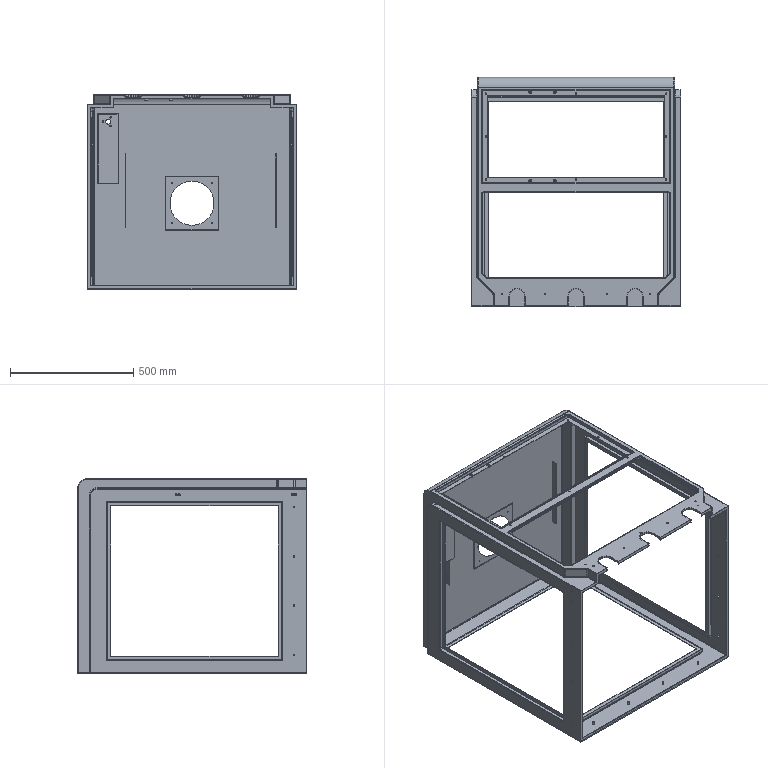Part | SolidWorks | features ICE 38, Fillet 16, HoleWzd 10, Chamfer 1, Cut 1, Extrusion 1, LPattern 1, Shell 1 | 11 solids | 563 faces | box 851 x 930 x 791 mm | volume 4286500 mm3 | cylinder 275 | plane 219 | torus 39 | cone 24 | sphere 4 | spline 2 | commonest cylinder face diameters 6 x107 8 x40 3.3 x32 2.5 x24 12 x18 10 x16